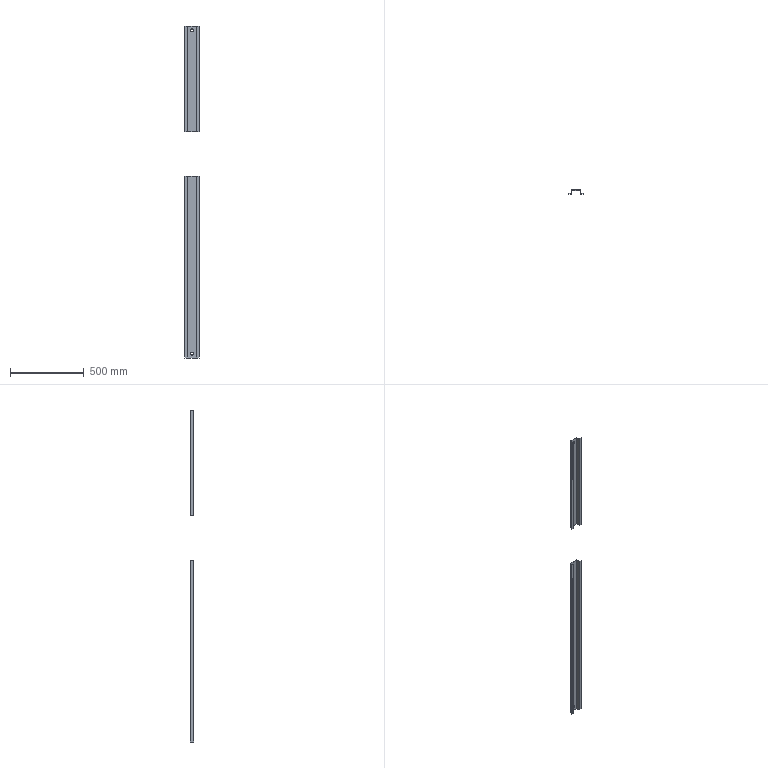Part | 2 solids | 80 faces | box 98.4 x 25 x 2251 mm | volume 224871 mm3 | plane 60 | cylinder 20 | commonest cylinder face diameters 2 x8 3.6 x8 20 x4